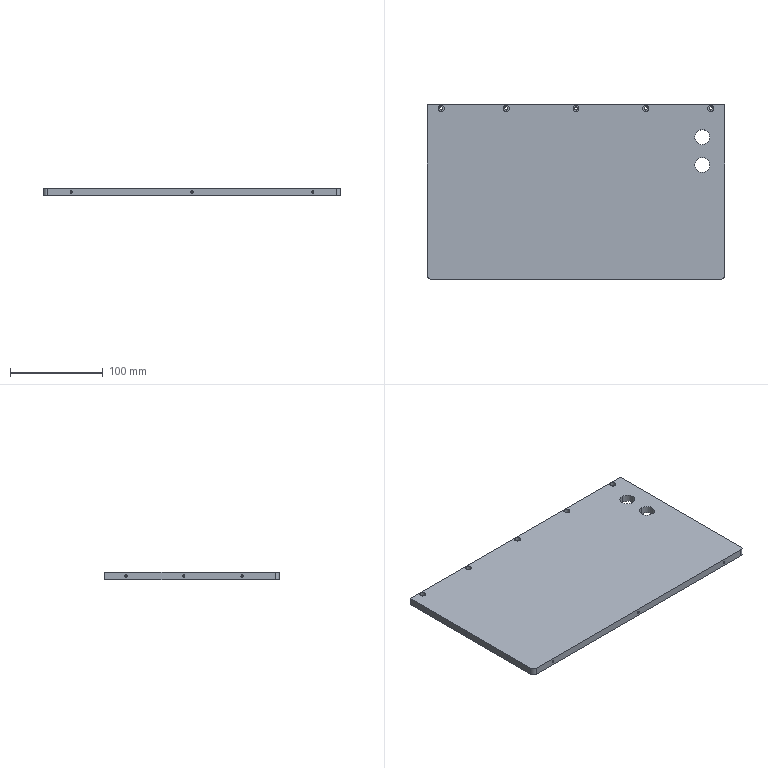NC program | Mastercam | posted with a generic post | part box 320 x 188 x 8 mm
Whole program:
%
O0000()
(MATERIAL - ALUMINUM MM - 2024)
( T1 | 10 FEM | H1 | XY STOCK TO LEAVE - .2 | Z STOCK TO LEAVE - 0. )
( T4 | 7.94 CTD | H4 )
( T5 | 3.4 DR | H5 )
( T6 | 4 FEM | H6 )
( T2 | 10 FEM | H2 | D2 | WEAR COMP | TOOL DIA. - 10. )
( T3 | 6 CHM | H3 )
N100 G21
N110 G0 G17 G40 G49 G80 G90
N120 T1 M6
N130 G0 G90 G54 X-167. Y105.2 A0. S8000 M3
N140 G43 H1 Z60.
N150 Z1.
N160 G1 Z-8. F600.
N170 Y103.2 F2000.
N180 G3 X-165. Y101.2 I2. J0.
N190 G1 X-160.
N200 X160.
N210 X165.
N220 G3 X167. Y103.2 I0. J2.
N230 G1 Y105.2
N240 G0 Z60.
N250 X-167. Y103.2
N260 Z1.
N270 G1 Z-8. F600.
N280 Y101.2 F2000.
N290 G3 X-165. Y99.2 I2. J0.
N300 G1 X-160.
N310 X160.
N320 X165.
N330 G3 X167. Y101.2 I0. J2.
N340 G1 Y103.2
N350 G0 Z60.
N360 X163. Y-105.2
N370 Z1.
N380 G1 Z-8. F600.
N390 Y-103.2 F2000.
N400 G3 X161. Y-101.2 I-2. J0.
N410 G1 X156.
N420 X-156.
N430 X-161.
N440 G3 X-163. Y-103.2 I0. J-2.
N450 G1 Y-105.2
N460 G0 Z60.
N470 X163. Y-103.2
N480 Z1.
N490 G1 Z-8. F600.
N500 Y-101.2 F2000.
N510 G3 X161. Y-99.2 I-2. J0.
N520 G1 X156.
N530 X-156.
N540 X-161.
N550 G3 X-163. Y-101.2 I0. J-2.
N560 G1 Y-103.2
N570 G0 Z60.
N580 M5
N590 G91 G28 Z0.
N600 A0.
N610 M01
N620 T4 M6
N630 G0 G90 G17 G54 X-145. Y90. A0. S2000 M3
N640 G43 H4 Z10.
N650 G98 G81 Z-1. R1. F200.
N660 X-75.
N670 X0.
N680 X75.
N690 X145.
N700 G80
N710 M5
N720 G91 G0 G28 Z0.
N730 A0.
N740 M01
N750 T5 M6
N760 G0 G90 G17 G54 X-145. Y90. A0. S1765 M3
N770 G43 H5 Z10.
N780 G98 G83 Z-10. R1. Q2. F200.
N790 X-75.
N800 X0.
N810 X75.
N820 X145.
N830 G80
N840 M5
N850 G91 G0 G28 Z0.
N860 A0.
N870 M01
N880 T6 M6
N890 G0 G90 G17 G54 X-145. Y91.25 A0. S8000 M3
N900 G43 H6 Z20.
N910 Z1.
N920 G1 Z.3 F600.
N930 G3 X-146.25 Y90. Z.175 I0. J-1.25 F1000.
N940 X-145. Y88.75 Z.05 I1.25 J0.
N950 X-143.75 Y90. Z-.075 I0. J1.25
N960 X-145. Y91.25 Z-.2 I-1.25 J0.
N970 X-146.25 Y90. Z-.325 I0. J-1.25
N980 X-145. Y88.75 Z-.45 I1.25 J0.
N990 X-143.75 Y90. Z-.575 I0. J1.25
N1000 X-145. Y91.25 Z-.7 I-1.25 J0.
N1010 X-146.25 Y90. Z-.825 I0. J-1.25
N1020 X-145. Y88.75 Z-.95 I1.25 J0.
N1030 X-143.75 Y90. Z-1.075 I0. J1.25
N1040 X-145. Y91.25 Z-1.2 I-1.25 J0.
N1050 X-146.25 Y90. Z-1.325 I0. J-1.25
N1060 X-145. Y88.75 Z-1.45 I1.25 J0.
N1070 X-143.75 Y90. Z-1.575 I0. J1.25
N1080 X-145. Y91.25 Z-1.7 I-1.25 J0.
N1090 X-146.25 Y90. Z-1.825 I0. J-1.25
N1100 X-145. Y88.75 Z-1.95 I1.25 J0.
N1110 X-143.75 Y90. Z-2.075 I0. J1.25
N1120 X-145. Y91.25 Z-2.2 I-1.25 J0.
N1130 X-146.25 Y90. Z-2.325 I0. J-1.25
N1140 X-145. Y88.75 Z-2.45 I1.25 J0.
N1150 X-143.75 Y90. Z-2.575 I0. J1.25
N1160 X-145. Y91.25 Z-2.7 I-1.25 J0.
N1170 X-146.25 Y90. Z-2.825 I0. J-1.25
N1180 X-145. Y88.75 Z-2.95 I1.25 J0.
N1190 X-143.75 Y90. Z-3.075 I0. J1.25
N1200 X-145. Y91.25 Z-3.2 I-1.25 J0.
N1210 X-146.25 Y90. Z-3.325 I0. J-1.25
N1220 X-145. Y88.75 Z-3.45 I1.25 J0.
N1230 X-143.75 Y90. Z-3.575 I0. J1.25
N1240 X-145. Y91.25 Z-3.7 I-1.25 J0.
N1250 X-146.25 Y90. Z-3.825 I0. J-1.25
N1260 X-145. Y88.75 Z-3.95 I1.25 J0.
N1270 X-144.265 Y88.989 Z-4. I0. J1.25
N1280 X-143.75 Y90. I-.735 J1.011
N1290 X-145. Y91.25 I-1.25 J0.
N1300 X-146.25 Y90. I0. J-1.25
N1310 X-145. Y88.75 I1.25 J0.
N1320 X-144.265 Y88.989 I0. J1.25
N1330 G0 Z20.
N1340 X-75. Y91.25
N1350 Z1.
N1360 G1 Z.3 F600.
N1370 G3 X-76.25 Y90. Z.175 I0. J-1.25 F1000.
N1380 X-75. Y88.75 Z.05 I1.25 J0.
N1390 X-73.75 Y90. Z-.075 I0. J1.25
N1400 X-75. Y91.25 Z-.2 I-1.25 J0.
N1410 X-76.25 Y90. Z-.325 I0. J-1.25
N1420 X-75. Y88.75 Z-.45 I1.25 J0.
N1430 X-73.75 Y90. Z-.575 I0. J1.25
N1440 X-75. Y91.25 Z-.7 I-1.25 J0.
N1450 X-76.25 Y90. Z-.825 I0. J-1.25
N1460 X-75. Y88.75 Z-.95 I1.25 J0.
N1470 X-73.75 Y90. Z-1.075 I0. J1.25
N1480 X-75. Y91.25 Z-1.2 I-1.25 J0.
N1490 X-76.25 Y90. Z-1.325 I0. J-1.25
N1500 X-75. Y88.75 Z-1.45 I1.25 J0.
N1510 X-73.75 Y90. Z-1.575 I0. J1.25
N1520 X-75. Y91.25 Z-1.7 I-1.25 J0.
N1530 X-76.25 Y90. Z-1.825 I0. J-1.25
N1540 X-75. Y88.75 Z-1.95 I1.25 J0.
N1550 X-73.75 Y90. Z-2.075 I0. J1.25
N1560 X-75. Y91.25 Z-2.2 I-1.25 J0.
N1570 X-76.25 Y90. Z-2.325 I0. J-1.25
N1580 X-75. Y88.75 Z-2.45 I1.25 J0.
N1590 X-73.75 Y90. Z-2.575 I0. J1.25
N1600 X-75. Y91.25 Z-2.7 I-1.25 J0.
N1610 X-76.25 Y90. Z-2.825 I0. J-1.25
N1620 X-75. Y88.75 Z-2.95 I1.25 J0.
N1630 X-73.75 Y90. Z-3.075 I0. J1.25
N1640 X-75. Y91.25 Z-3.2 I-1.25 J0.
N1650 X-76.25 Y90. Z-3.325 I0. J-1.25
N1660 X-75. Y88.75 Z-3.45 I1.25 J0.
N1670 X-73.75 Y90. Z-3.575 I0. J1.25
N1680 X-75. Y91.25 Z-3.7 I-1.25 J0.
N1690 X-76.25 Y90. Z-3.825 I0. J-1.25
N1700 X-75. Y88.75 Z-3.95 I1.25 J0.
N1710 X-74.265 Y88.989 Z-4. I0. J1.25
N1720 X-73.75 Y90. I-.735 J1.011
N1730 X-75. Y91.25 I-1.25 J0.
N1740 X-76.25 Y90. I0. J-1.25
N1750 X-75. Y88.75 I1.25 J0.
N1760 X-74.265 Y88.989 I0. J1.25
N1770 G0 Z20.
N1780 X0. Y91.25
N1790 Z1.
N1800 G1 Z.3 F600.
N1810 G3 X-1.25 Y90. Z.175 I0. J-1.25 F1000.
N1820 X0. Y88.75 Z.05 I1.25 J0.
N1830 X1.25 Y90. Z-.075 I0. J1.25
N1840 X0. Y91.25 Z-.2 I-1.25 J0.
N1850 X-1.25 Y90. Z-.325 I0. J-1.25
N1860 X0. Y88.75 Z-.45 I1.25 J0.
N1870 X1.25 Y90. Z-.575 I0. J1.25
N1880 X0. Y91.25 Z-.7 I-1.25 J0.
N1890 X-1.25 Y90. Z-.825 I0. J-1.25
N1900 X0. Y88.75 Z-.95 I1.25 J0.
N1910 X1.25 Y90. Z-1.075 I0. J1.25
N1920 X0. Y91.25 Z-1.2 I-1.25 J0.
N1930 X-1.25 Y90. Z-1.325 I0. J-1.25
N1940 X0. Y88.75 Z-1.45 I1.25 J0.
N1950 X1.25 Y90. Z-1.575 I0. J1.25
N1960 X0. Y91.25 Z-1.7 I-1.25 J0.
N1970 X-1.25 Y90. Z-1.825 I0. J-1.25
N1980 X0. Y88.75 Z-1.95 I1.25 J0.
N1990 X1.25 Y90. Z-2.075 I0. J1.25
N2000 X0. Y91.25 Z-2.2 I-1.25 J0.
N2010 X-1.25 Y90. Z-2.325 I0. J-1.25
N2020 X0. Y88.75 Z-2.45 I1.25 J0.
N2030 X1.25 Y90. Z-2.575 I0. J1.25
N2040 X0. Y91.25 Z-2.7 I-1.25 J0.
N2050 X-1.25 Y90. Z-2.825 I0. J-1.25
N2060 X0. Y88.75 Z-2.95 I1.25 J0.
N2070 X1.25 Y90. Z-3.075 I0. J1.25
N2080 X0. Y91.25 Z-3.2 I-1.25 J0.
N2090 X-1.25 Y90. Z-3.325 I0. J-1.25
N2100 X0. Y88.75 Z-3.45 I1.25 J0.
N2110 X1.25 Y90. Z-3.575 I0. J1.25
N2120 X0. Y91.25 Z-3.7 I-1.25 J0.
N2130 X-1.25 Y90. Z-3.825 I0. J-1.25
N2140 X0. Y88.75 Z-3.95 I1.25 J0.
N2150 X.735 Y88.989 Z-4. I0. J1.25
N2160 X1.25 Y90. I-.735 J1.011
N2170 X0. Y91.25 I-1.25 J0.
N2180 X-1.25 Y90. I0. J-1.25
N2190 X0. Y88.75 I1.25 J0.
N2200 X.735 Y88.989 I0. J1.25
N2210 G0 Z20.
N2220 X75. Y91.25
N2230 Z1.
N2240 G1 Z.3 F600.
N2250 G3 X73.75 Y90. Z.175 I0. J-1.25 F1000.
N2260 X75. Y88.75 Z.05 I1.25 J0.
N2270 X76.25 Y90. Z-.075 I0. J1.25
N2280 X75. Y91.25 Z-.2 I-1.25 J0.
N2290 X73.75 Y90. Z-.325 I0. J-1.25
N2300 X75. Y88.75 Z-.45 I1.25 J0.
N2310 X76.25 Y90. Z-.575 I0. J1.25
N2320 X75. Y91.25 Z-.7 I-1.25 J0.
N2330 X73.75 Y90. Z-.825 I0. J-1.25
N2340 X75. Y88.75 Z-.95 I1.25 J0.
N2350 X76.25 Y90. Z-1.075 I0. J1.25
N2360 X75. Y91.25 Z-1.2 I-1.25 J0.
N2370 X73.75 Y90. Z-1.325 I0. J-1.25
N2380 X75. Y88.75 Z-1.45 I1.25 J0.
N2390 X76.25 Y90. Z-1.575 I0. J1.25
N2400 X75. Y91.25 Z-1.7 I-1.25 J0.
N2410 X73.75 Y90. Z-1.825 I0. J-1.25
N2420 X75. Y88.75 Z-1.95 I1.25 J0.
N2430 X76.25 Y90. Z-2.075 I0. J1.25
N2440 X75. Y91.25 Z-2.2 I-1.25 J0.
N2450 X73.75 Y90. Z-2.325 I0. J-1.25
N2460 X75. Y88.75 Z-2.45 I1.25 J0.
N2470 X76.25 Y90. Z-2.575 I0. J1.25
N2480 X75. Y91.25 Z-2.7 I-1.25 J0.
N2490 X73.75 Y90. Z-2.825 I0. J-1.25
N2500 X75. Y88.75 Z-2.95 I1.25 J0.
N2510 X76.25 Y90. Z-3.075 I0. J1.25
N2520 X75. Y91.25 Z-3.2 I-1.25 J0.
N2530 X73.75 Y90. Z-3.325 I0. J-1.25
N2540 X75. Y88.75 Z-3.45 I1.25 J0.
N2550 X76.25 Y90. Z-3.575 I0. J1.25
N2560 X75. Y91.25 Z-3.7 I-1.25 J0.
N2570 X73.75 Y90. Z-3.825 I0. J-1.25
N2580 X75. Y88.75 Z-3.95 I1.25 J0.
N2590 X75.735 Y88.989 Z-4. I0. J1.25
N2600 X76.25 Y90. I-.735 J1.011
N2610 X75. Y91.25 I-1.25 J0.
N2620 X73.75 Y90. I0. J-1.25
N2630 X75. Y88.75 I1.25 J0.
N2640 X75.735 Y88.989 I0. J1.25
N2650 G0 Z20.
N2660 X145. Y91.25
N2670 Z1.
N2680 G1 Z.3 F600.
N2690 G3 X143.75 Y90. Z.175 I0. J-1.25 F1000.
N2700 X145. Y88.75 Z.05 I1.25 J0.
N2710 X146.25 Y90. Z-.075 I0. J1.25
N2720 X145. Y91.25 Z-.2 I-1.25 J0.
N2730 X143.75 Y90. Z-.325 I0. J-1.25
N2740 X145. Y88.75 Z-.45 I1.25 J0.
N2750 X146.25 Y90. Z-.575 I0. J1.25
N2760 X145. Y91.25 Z-.7 I-1.25 J0.
N2770 X143.75 Y90. Z-.825 I0. J-1.25
N2780 X145. Y88.75 Z-.95 I1.25 J0.
N2790 X146.25 Y90. Z-1.075 I0. J1.25
N2800 X145. Y91.25 Z-1.2 I-1.25 J0.
N2810 X143.75 Y90. Z-1.325 I0. J-1.25
N2820 X145. Y88.75 Z-1.45 I1.25 J0.
N2830 X146.25 Y90. Z-1.575 I0. J1.25
N2840 X145. Y91.25 Z-1.7 I-1.25 J0.
N2850 X143.75 Y90. Z-1.825 I0. J-1.25
N2860 X145. Y88.75 Z-1.95 I1.25 J0.
N2870 X146.25 Y90. Z-2.075 I0. J1.25
N2880 X145. Y91.25 Z-2.2 I-1.25 J0.
N2890 X143.75 Y90. Z-2.325 I0. J-1.25
N2900 X145. Y88.75 Z-2.45 I1.25 J0.
N2910 X146.25 Y90. Z-2.575 I0. J1.25
N2920 X145. Y91.25 Z-2.7 I-1.25 J0.
N2930 X143.75 Y90. Z-2.825 I0. J-1.25
N2940 X145. Y88.75 Z-2.95 I1.25 J0.
N2950 X146.25 Y90. Z-3.075 I0. J1.25
N2960 X145. Y91.25 Z-3.2 I-1.25 J0.
N2970 X143.75 Y90. Z-3.325 I0. J-1.25
N2980 X145. Y88.75 Z-3.45 I1.25 J0.
N2990 X146.25 Y90. Z-3.575 I0. J1.25
N3000 X145. Y91.25 Z-3.7 I-1.25 J0.
N3010 X143.75 Y90. Z-3.825 I0. J-1.25
N3020 X145. Y88.75 Z-3.95 I1.25 J0.
N3030 X145.735 Y88.989 Z-4. I0. J1.25
N3040 X146.25 Y90. I-.735 J1.011
N3050 X145. Y91.25 I-1.25 J0.
N3060 X143.75 Y90. I0. J-1.25
N3070 X145. Y88.75 I1.25 J0.
N3080 X145.735 Y88.989 I0. J1.25
N3090 G0 Z20.
N3100 M5
N3110 G91 G28 Z0.
N3120 A0.
N3130 M01
N3140 T2 M6
N3150 G0 G90 G17 G54 X-165.3 Y99.6 A0. S8000 M3
N3160 G43 H2 Z60.
N3170 Z1.
N3180 G1 Z-8. F600.
N3190 G41 D2 Y99.3 F1000.
N3200 G3 X-165. Y99. I.3 J0.
N3210 G1 X-160.
N3220 X160.
N3230 X165.
N3240 G3 X165.3 Y99.3 I0. J.3
N3250 G1 G40 Y99.6
N3260 G0 Z60.
N3270 X161.3 Y-99.6
N3280 Z1.
N3290 G1 Z-8. F600.
N3300 G41 D2 Y-99.3 F1000.
N3310 G3 X161. Y-99. I-.3 J0.
N3320 G1 X156.
N3330 X-156.
N3340 X-161.
N3350 G3 X-161.3 Y-99.3 I0. J-.3
N3360 G1 G40 Y-99.6
N3370 G0 Z60.
N3380 M5
N3390 G91 G28 Z0.
N3400 A0.
N3410 M01
N3420 T3 M6
N3430 G0 G90 G17 G54 X156.3 Y-95.75 A0. S5000 M3
N3440 G43 H3 Z60.
N3450 Z59.5
N3460 Z-.5
N3470 G1 Z-1.5 F600.
N3480 Y-95.45 F1000.
N3490 G3 X156. Y-95.15 I-.3 J0.
N3500 G1 X-156.
N3510 G3 X-156.3 Y-95.45 I0. J-.3
N3520 G1 Y-95.75
N3530 G0 Z58.5
N3540 Z60.
N3550 X-144.7 Y91.5
N3560 Z59.5
N3570 Z-.5
N3580 G1 Z-1.5 F600.
N3590 Y91.8 F1000.
N3600 G3 X-145. Y92.1 I-.3 J0.
N3610 X-147.1 Y90. I0. J-2.1
N3620 X-145. Y87.9 I2.1 J0.
N3630 X-142.9 Y90. I0. J2.1
N3640 X-145. Y92.1 I-2.1 J0.
N3650 X-145.3 Y91.8 I0. J-.3
N3660 G1 Y91.5
N3670 G0 Z58.5
N3680 Z60.
N3690 X-152.8 Y93.625
N3700 X-160.3 Y95.75
N3710 Z59.5
N3720 Z-.5
N3730 G1 Z-1.5 F600.
N3740 Y95.45 F1000.
N3750 G3 X-160. Y95.15 I.3 J0.
N3760 G1 X160.
N3770 G3 X160.3 Y95.45 I0. J.3
N3780 G1 Y95.75
N3790 G0 Z58.5
N3800 Z60.
N3810 X152.8 Y93.625
N3820 X145.3 Y91.5
N3830 Z59.5
N3840 Z-.5
N3850 G1 Z-1.5 F600.
N3860 Y91.8 F1000.
N3870 G3 X145. Y92.1 I-.3 J0.
N3880 X142.9 Y90. I0. J-2.1
N3890 X145. Y87.9 I2.1 J0.
N3900 X147.1 Y90. I0. J2.1
N3910 X145. Y92.1 I-2.1 J0.
N3920 X144.7 Y91.8 I0. J-.3
N3930 G1 Y91.5
N3940 G0 Z58.5
N3950 Z60.
N3960 X75.3
N3970 Z59.5
N3980 Z-.5
N3990 G1 Z-1.5 F600.
N4000 Y91.8 F1000.
N4010 G3 X75. Y92.1 I-.3 J0.
N4020 X72.9 Y90. I0. J-2.1
N4030 X75. Y87.9 I2.1 J0.
N4040 X77.1 Y90. I0. J2.1
N4050 X75. Y92.1 I-2.1 J0.
N4060 X74.7 Y91.8 I0. J-.3
N4070 G1 Y91.5
N4080 G0 Z58.5
N4090 Z60.
N4100 X37.5
N4110 X.3
N4120 Z59.5
N4130 Z-.5
N4140 G1 Z-1.5 F600.
N4150 Y91.8 F1000.
N4160 G3 X0. Y92.1 I-.3 J0.
N4170 X-2.1 Y90. I0. J-2.1
N4180 X0. Y87.9 I2.1 J0.
N4190 X2.1 Y90. I0. J2.1
N4200 X0. Y92.1 I-2.1 J0.
N4210 X-.3 Y91.8 I0. J-.3
N4220 G1 Y91.5
N4230 G0 Z58.5
N4240 Z60.
N4250 X-37.5
N4260 X-74.7
N4270 Z59.5
N4280 Z-.5
N4290 G1 Z-1.5 F600.
N4300 Y91.8 F1000.
N4310 G3 X-75. Y92.1 I-.3 J0.
N4320 X-77.1 Y90. I0. J-2.1
N4330 X-75. Y87.9 I2.1 J0.
N4340 X-72.9 Y90. I0. J2.1
N4350 X-75. Y92.1 I-2.1 J0.
N4360 X-75.3 Y91.8 I0. J-.3
N4370 G1 Y91.5
N4380 G0 Z58.5
N4390 Z60.
N4400 M5
N4410 G91 G28 Z0.
N4420 G28 X0. Y0. A0.
N4430 M30
%